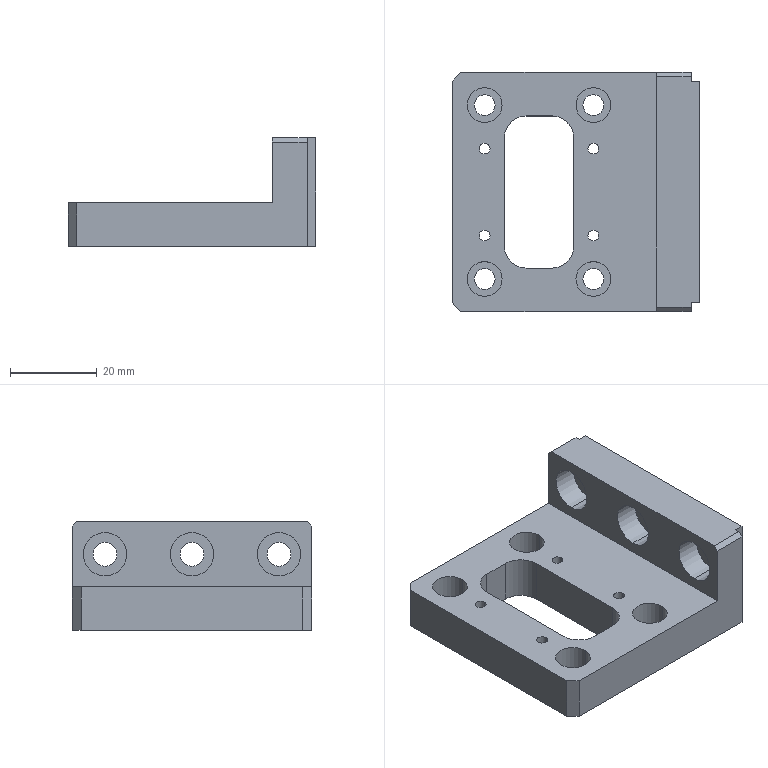Part | SolidWorks | features HoleWzd 3, ICE 3, Chamfer 2, Extrusion 1, Fillet 1 | 1 solid | 67 faces | box 57 x 55 x 25 mm | volume 30548 mm3 | cylinder 40 | plane 27 | commonest cylinder face diameters 10 x10 2.5 x8 4.8 x8 8 x8 5.5 x6